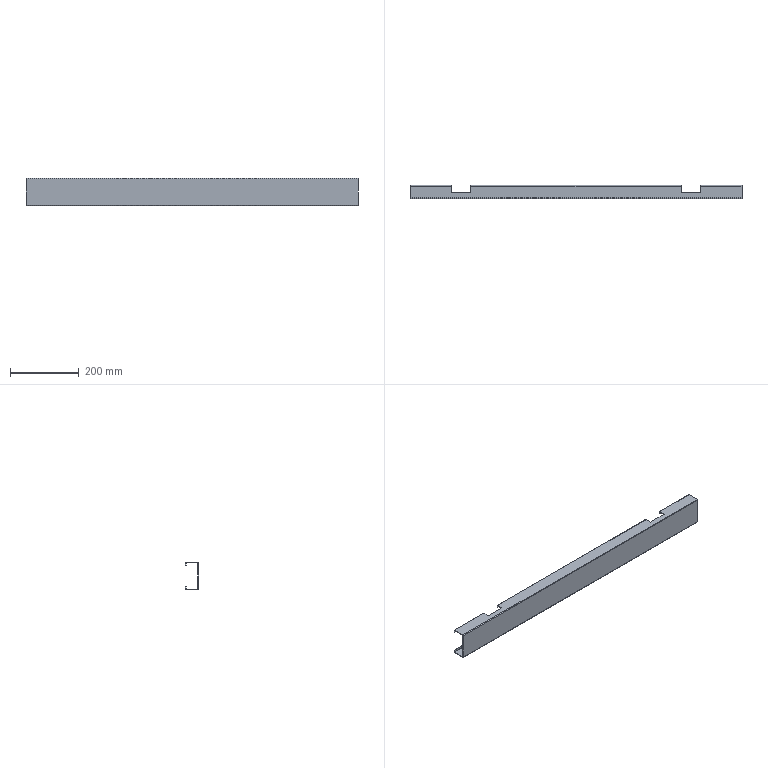Part | SolidWorks | features FlatPattern 1, ICE 1, SMBaseFlange 1, SheetMetal 1 | 1 solid | 86 faces | box 969 x 38 x 80 mm | volume 230143 mm3 | plane 70 | cylinder 16 | commonest cylinder face diameters 0.4 x8 3.4 x8